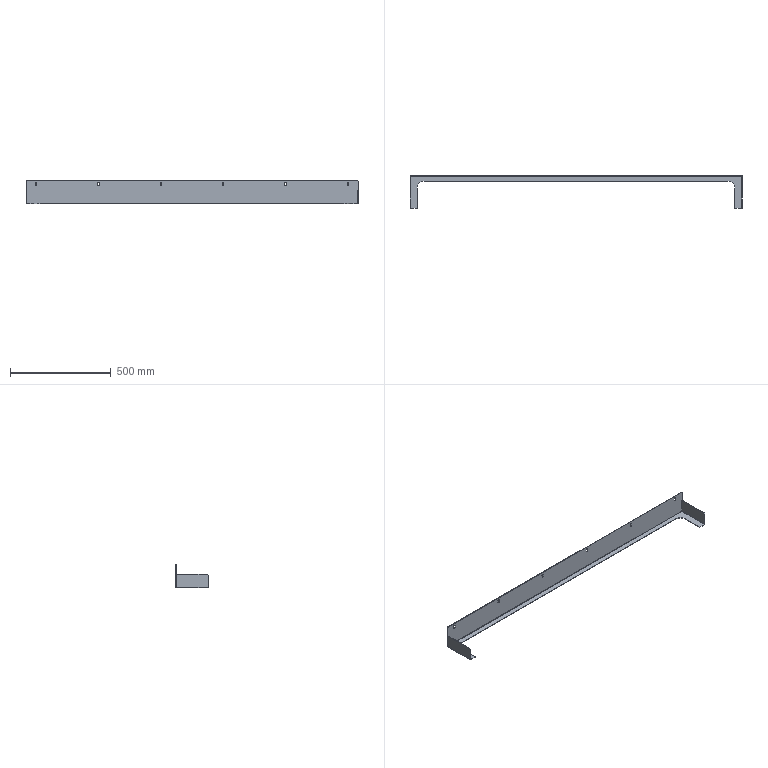Part | STEP file | 1 solid | 64 faces | box 1650 x 162 x 118 mm | volume 529354 mm3 | plane 36 | cylinder 28 | commonest cylinder face diameters 8 x18 2 x3 6 x3 10 x2 70 x2